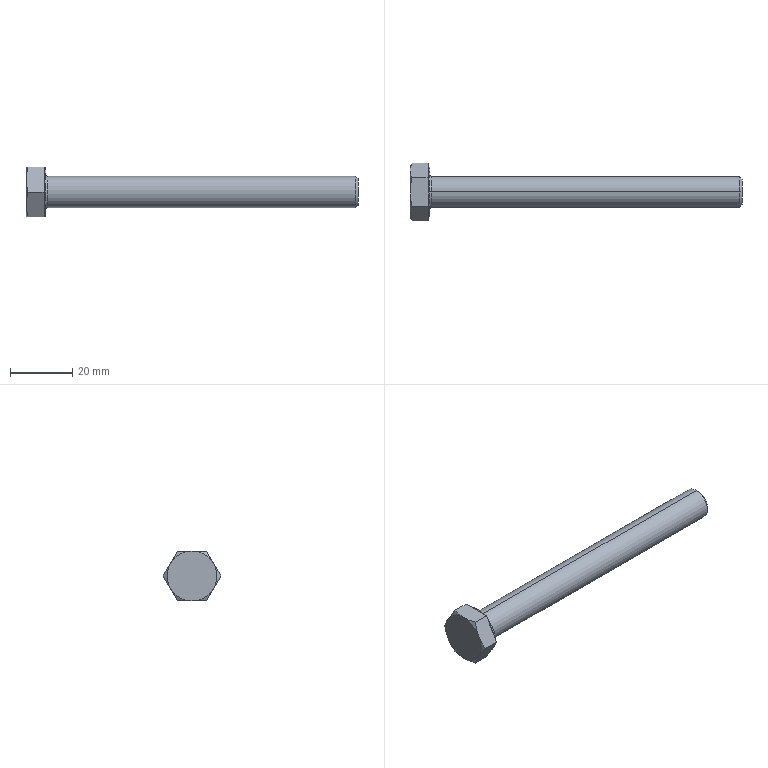Part | STEP file | Microwave Drying Flat Conveyor-hex screw gradeab_din_DIN EN 24017 - M10 x 100-N_Default | 1 solid | 29 faces | box 106.4 x 18.475 x 16 mm | volume 9247 mm3 | plane 15 | cone 8 | cylinder 4 | spline 2 | commonest cylinder face diameters 10 x2 16 x2
STEP:
#1=CARTESIAN_POINT('',(6.4,0.,5.4));
#2=VERTEX_POINT('',#1);
#3=CARTESIAN_POINT('',(6.4,0.,-5.4));
#4=VERTEX_POINT('',#3);
#5=CARTESIAN_POINT('',(6.4,0.,5.4));
#6=CARTESIAN_POINT('',(6.4,0.1651,5.4));
#7=CARTESIAN_POINT('',(6.4,0.4117,5.389));
#8=CARTESIAN_POINT('',(6.4,0.6977,5.356));
#9=CARTESIAN_POINT('',(6.4,0.8403,5.334));
#10=CARTESIAN_POINT('',(6.4,0.9013,5.324));
#11=CARTESIAN_POINT('',(6.4,0.942,5.317));
#12=CARTESIAN_POINT('',(6.4,0.9611,5.314));
#13=CARTESIAN_POINT('',(6.4,1.155,5.278));
#14=CARTESIAN_POINT('',(6.4,1.409,5.218));
#15=CARTESIAN_POINT('',(6.4,1.7,5.127));
#16=CARTESIAN_POINT('',(6.4,1.824,5.083));
#17=CARTESIAN_POINT('',(6.4,1.906,5.053));
#18=CARTESIAN_POINT('',(6.4,1.945,5.038));
#19=CARTESIAN_POINT('',(6.4,2.157,4.954));
#20=CARTESIAN_POINT('',(6.4,2.405,4.841));
#21=CARTESIAN_POINT('',(6.4,2.644,4.709));
#22=CARTESIAN_POINT('',(6.4,2.801,4.618));
#23=CARTESIAN_POINT('',(6.4,2.877,4.571));
#24=CARTESIAN_POINT('',(6.4,3.267,4.316));
#25=CARTESIAN_POINT('',(6.4,3.555,4.082));
#26=CARTESIAN_POINT('',(6.4,3.95,3.687));
#27=CARTESIAN_POINT('',(6.4,4.137,3.48));
#28=CARTESIAN_POINT('',(6.4,4.306,3.26));
#29=CARTESIAN_POINT('',(6.4,4.416,3.11));
#30=CARTESIAN_POINT('',(6.4,4.47,3.031));
#31=CARTESIAN_POINT('',(6.4,4.62,2.802));
#32=CARTESIAN_POINT('',(6.4,4.757,2.567));
#33=CARTESIAN_POINT('',(6.4,4.896,2.281));
#34=CARTESIAN_POINT('',(6.4,4.951,2.156));
#35=CARTESIAN_POINT('',(6.4,4.987,2.072));
#36=CARTESIAN_POINT('',(6.4,5.005,2.028));
#37=CARTESIAN_POINT('',(6.4,5.085,1.825));
#38=CARTESIAN_POINT('',(6.4,5.17,1.577));
#39=CARTESIAN_POINT('',(6.4,5.247,1.282));
#40=CARTESIAN_POINT('',(6.4,5.28,1.133));
#41=CARTESIAN_POINT('',(6.4,5.293,1.069));
#42=CARTESIAN_POINT('',(6.4,5.302,1.026));
#43=CARTESIAN_POINT('',(6.4,5.306,1.003));
#44=CARTESIAN_POINT('',(6.4,5.37,0.6582));
#45=CARTESIAN_POINT('',(6.4,5.4,0.3299));
#46=CARTESIAN_POINT('',(6.4,5.4,-0.165));
#47=CARTESIAN_POINT('',(6.4,5.389,-0.4115));
#48=CARTESIAN_POINT('',(6.4,5.356,-0.6976));
#49=CARTESIAN_POINT('',(6.4,5.335,-0.8402));
#50=CARTESIAN_POINT('',(6.4,5.324,-0.9013));
#51=CARTESIAN_POINT('',(6.4,5.317,-0.9419));
#52=CARTESIAN_POINT('',(6.4,5.314,-0.9611));
#53=CARTESIAN_POINT('',(6.4,5.278,-1.155));
#54=CARTESIAN_POINT('',(6.4,5.218,-1.409));
#55=CARTESIAN_POINT('',(6.4,5.127,-1.7));
#56=CARTESIAN_POINT('',(6.4,5.083,-1.824));
#57=CARTESIAN_POINT('',(6.4,5.053,-1.906));
#58=CARTESIAN_POINT('',(6.4,5.038,-1.945));
#59=CARTESIAN_POINT('',(6.4,4.954,-2.157));
#60=CARTESIAN_POINT('',(6.4,4.841,-2.405));
#61=CARTESIAN_POINT('',(6.4,4.709,-2.644));
#62=CARTESIAN_POINT('',(6.4,4.618,-2.801));
#63=CARTESIAN_POINT('',(6.4,4.571,-2.877));
#64=CARTESIAN_POINT('',(6.4,4.316,-3.267));
#65=CARTESIAN_POINT('',(6.4,4.082,-3.555));
#66=CARTESIAN_POINT('',(6.4,3.687,-3.95));
#67=CARTESIAN_POINT('',(6.4,3.48,-4.137));
#68=CARTESIAN_POINT('',(6.4,3.26,-4.306));
#69=CARTESIAN_POINT('',(6.4,3.11,-4.416));
#70=CARTESIAN_POINT('',(6.4,3.031,-4.47));
#71=CARTESIAN_POINT('',(6.4,2.802,-4.62));
#72=CARTESIAN_POINT('',(6.4,2.567,-4.757));
#73=CARTESIAN_POINT('',(6.4,2.281,-4.896));
#74=CARTESIAN_POINT('',(6.4,2.156,-4.951));
#75=CARTESIAN_POINT('',(6.4,2.072,-4.987));
#76=CARTESIAN_POINT('',(6.4,2.028,-5.005));
#77=CARTESIAN_POINT('',(6.4,1.825,-5.085));
#78=CARTESIAN_POINT('',(6.4,1.577,-5.17));
#79=CARTESIAN_POINT('',(6.4,1.282,-5.247));
#80=CARTESIAN_POINT('',(6.4,1.133,-5.28));
#81=CARTESIAN_POINT('',(6.4,1.069,-5.293));
#82=CARTESIAN_POINT('',(6.4,1.026,-5.302));
#83=CARTESIAN_POINT('',(6.4,1.003,-5.306));
#84=CARTESIAN_POINT('',(6.4,0.658,-5.37));
#85=CARTESIAN_POINT('',(6.4,0.3305,-5.4));
#86=CARTESIAN_POINT('',(6.4,0.,-5.4));
#87=B_SPLINE_CURVE_WITH_KNOTS('',3,(#5,#6,#7,#8,#9,#10,#11,#12,#13,#14,#15,#16,#17,#18,#19,#20,#21,#22,#23,#24,#25,#26,#27,#28,#29,#30,#31,#32,#33,#34,#35,#36,#37,#38,#39,#40,#41,#42,#43,#44,#45,#46,#47,#48,#49,#50,#51,#52,#53,#54,#55,#56,#57,#58,#59,#60,#61,#62,#63,#64,#65,#66,#67,#68,#69,#70,#71,#72,#73,#74,#75,#76,#77,#78,#79,#80,#81,#82,#83,#84,#85,#86),.UNSPECIFIED.,.F.,.F.,(4,1,1,1,2,2,1,1,2,2,1,2,2,2,1,2,2,1,1,2,2,1,1,1,2,2,2,1,1,1,2,2,1,1,2,2,1,2,2,2,1,2,2,1,1,2,2,1,1,1,2,2,4),(0.,0.03125,0.04687,0.05469,0.05859,0.0625,0.09375,0.1094,0.1172,0.125,0.1562,0.1719,0.1875,0.25,0.2812,0.2969,0.3125,0.3437,0.3594,0.3672,0.375,0.4062,0.4219,0.4297,0.4336,0.4375,0.5,0.5312,0.5469,0.5547,0.5586,0.5625,0.5937,0.6094,0.6172,0.625,0.6562,0.6719,0.6875,0.75,0.7812,0.7969,0.8125,0.8437,0.8594,0.8672,0.875,0.9062,0.9219,0.9297,0.9336,0.9375,1.),.UNSPECIFIED.);
#88=EDGE_CURVE('',#2,#4,#87,.T.);
#89=ORIENTED_EDGE('',*,*,#88,.F.);
#90=CARTESIAN_POINT('',(6.8,0.,5.));
#91=VERTEX_POINT('',#90);
#92=CARTESIAN_POINT('',(6.8,0.,5.4));
#93=DIRECTION('',(0.,-1.,0.));
#94=DIRECTION('',(0.,0.,1.));
#95=AXIS2_PLACEMENT_3D('',#92,#93,#94);
#96=CIRCLE('',#95,0.4);
#97=EDGE_CURVE('',#2,#91,#96,.T.);
#98=ORIENTED_EDGE('',*,*,#97,.T.);
#99=CARTESIAN_POINT('',(6.8,0.,-5.));
#100=VERTEX_POINT('',#99);
#101=CARTESIAN_POINT('',(6.8,0.,0.));
#102=DIRECTION('',(1.,0.,0.));
#103=DIRECTION('',(0.,0.,1.));
#104=AXIS2_PLACEMENT_3D('',#101,#102,#103);
#105=CIRCLE('',#104,5.);
#106=EDGE_CURVE('',#100,#91,#105,.T.);
#107=ORIENTED_EDGE('',*,*,#106,.F.);
#108=CARTESIAN_POINT('',(6.8,0.,-5.4));
#109=DIRECTION('',(0.,1.,0.));
#110=DIRECTION('',(0.,0.,-1.));
#111=AXIS2_PLACEMENT_3D('',#108,#109,#110);
#112=CIRCLE('',#111,0.4);
#113=EDGE_CURVE('',#4,#100,#112,.T.);
#114=ORIENTED_EDGE('',*,*,#113,.F.);
#115=EDGE_LOOP('',(#89,#98,#107,#114));
#116=FACE_OUTER_BOUND('',#115,.T.);
#117=CARTESIAN_POINT('',(6.4,0.,-5.4));
#118=CARTESIAN_POINT('',(6.4,10.8,-5.4));
#119=CARTESIAN_POINT('',(6.4,10.8,5.4));
#120=CARTESIAN_POINT('',(6.4,0.,5.4));
#121=CARTESIAN_POINT('',(6.4,0.,-5.166));
#122=CARTESIAN_POINT('',(6.4,10.331,-5.166));
#123=CARTESIAN_POINT('',(6.4,10.331,5.166));
#124=CARTESIAN_POINT('',(6.4,0.,5.166));
#125=CARTESIAN_POINT('',(6.566,0.,-5.));
#126=CARTESIAN_POINT('',(6.566,10.,-5.));
#127=CARTESIAN_POINT('',(6.566,10.,5.));
#128=CARTESIAN_POINT('',(6.566,0.,5.));
#129=CARTESIAN_POINT('',(6.8,0.,-5.));
#130=CARTESIAN_POINT('',(6.8,10.,-5.));
#131=CARTESIAN_POINT('',(6.8,10.,5.));
#132=CARTESIAN_POINT('',(6.8,0.,5.));
#133=(BOUNDED_SURFACE()B_SPLINE_SURFACE(3,3,((#117,#118,#119,#120),(#121,#122,#123,#124),(#125,#126,#127,#128),(#129,#130,#131,#132)),.UNSPECIFIED.,.F.,.F.,.F.)B_SPLINE_SURFACE_WITH_KNOTS((4,4),(4,4),(0.,1.),(0.,1.),.UNSPECIFIED.)GEOMETRIC_REPRESENTATION_ITEM()RATIONAL_B_SPLINE_SURFACE(((1.,0.3333,0.3333,1.),(0.8047,0.2682,0.2682,0.8047),(0.8047,0.2682,0.2682,0.8047),(1.,0.3333,0.3333,1.)))REPRESENTATION_ITEM('')SURFACE());
#134=ADVANCED_FACE('',(#116),#133,.F.);
#135=CARTESIAN_POINT('',(105.572,0.,5.));
#136=VERTEX_POINT('',#135);
#137=CARTESIAN_POINT('',(105.572,0.,-5.));
#138=VERTEX_POINT('',#137);
#139=CARTESIAN_POINT('',(105.572,0.,0.));
#140=DIRECTION('',(-1.,0.,0.));
#141=DIRECTION('',(0.,0.,1.));
#142=AXIS2_PLACEMENT_3D('',#139,#140,#141);
#143=CIRCLE('',#142,5.);
#144=EDGE_CURVE('',#136,#138,#143,.T.);
#145=ORIENTED_EDGE('',*,*,#144,.T.);
#146=CARTESIAN_POINT('',(0.,0.,-5.));
#147=DIRECTION('',(-1.,0.,0.));
#148=VECTOR('',#147,1000.);
#149=LINE('',#146,#148);
#150=EDGE_CURVE('',#138,#100,#149,.T.);
#151=ORIENTED_EDGE('',*,*,#150,.T.);
#152=ORIENTED_EDGE('',*,*,#106,.T.);
#153=CARTESIAN_POINT('',(0.,0.,5.));
#154=DIRECTION('',(-1.,0.,0.));
#155=VECTOR('',#154,1000.);
#156=LINE('',#153,#155);
#157=EDGE_CURVE('',#136,#91,#156,.T.);
#158=ORIENTED_EDGE('',*,*,#157,.F.);
#159=EDGE_LOOP('',(#145,#151,#152,#158));
#160=FACE_OUTER_BOUND('',#159,.T.);
#161=CARTESIAN_POINT('',(0.,0.,0.));
#162=DIRECTION('',(-1.,0.,0.));
#163=DIRECTION('',(0.,0.,1.));
#164=AXIS2_PLACEMENT_3D('',#161,#162,#163);
#165=CYLINDRICAL_SURFACE('',#164,5.);
#166=ADVANCED_FACE('',(#160),#165,.T.);
#167=CARTESIAN_POINT('',(106.4,0.,4.172));
#168=VERTEX_POINT('',#167);
#169=CARTESIAN_POINT('',(106.4,0.,-4.172));
#170=VERTEX_POINT('',#169);
#171=CARTESIAN_POINT('',(106.4,0.,0.));
#172=DIRECTION('',(-1.,0.,0.));
#173=DIRECTION('',(0.,0.,1.));
#174=AXIS2_PLACEMENT_3D('',#171,#172,#173);
#175=CIRCLE('',#174,4.172);
#176=EDGE_CURVE('',#168,#170,#175,.T.);
#177=ORIENTED_EDGE('',*,*,#176,.T.);
#178=CARTESIAN_POINT('',(105.572,0.,-5.));
#179=DIRECTION('',(-0.7071,0.,-0.7071));
#180=VECTOR('',#179,1000.);
#181=LINE('',#178,#180);
#182=EDGE_CURVE('',#170,#138,#181,.T.);
#183=ORIENTED_EDGE('',*,*,#182,.T.);
#184=ORIENTED_EDGE('',*,*,#144,.F.);
#185=CARTESIAN_POINT('',(105.572,0.,5.));
#186=DIRECTION('',(-0.7071,0.,0.7071));
#187=VECTOR('',#186,1000.);
#188=LINE('',#185,#187);
#189=EDGE_CURVE('',#168,#136,#188,.T.);
#190=ORIENTED_EDGE('',*,*,#189,.F.);
#191=EDGE_LOOP('',(#177,#183,#184,#190));
#192=FACE_OUTER_BOUND('',#191,.T.);
#193=CARTESIAN_POINT('',(105.572,0.,0.));
#194=DIRECTION('',(-1.,0.,0.));
#195=DIRECTION('',(0.,0.,1.));
#196=AXIS2_PLACEMENT_3D('',#193,#194,#195);
#197=CONICAL_SURFACE('',#196,5.,0.7854);
#198=ADVANCED_FACE('',(#192),#197,.T.);
#199=CARTESIAN_POINT('',(6.4,0.,-8.));
#200=VERTEX_POINT('',#199);
#201=CARTESIAN_POINT('',(6.4,0.,8.));
#202=VERTEX_POINT('',#201);
#203=CARTESIAN_POINT('',(6.4,0.,0.));
#204=DIRECTION('',(1.,0.,0.));
#205=DIRECTION('',(0.,0.,1.));
#206=AXIS2_PLACEMENT_3D('',#203,#204,#205);
#207=CIRCLE('',#206,8.);
#208=EDGE_CURVE('',#200,#202,#207,.T.);
#209=ORIENTED_EDGE('',*,*,#208,.F.);
#210=CARTESIAN_POINT('',(5.8,0.,-8.));
#211=VERTEX_POINT('',#210);
#212=CARTESIAN_POINT('',(0.,0.,-8.));
#213=DIRECTION('',(-1.,0.,0.));
#214=VECTOR('',#213,1000.);
#215=LINE('',#212,#214);
#216=EDGE_CURVE('',#200,#211,#215,.T.);
#217=ORIENTED_EDGE('',*,*,#216,.T.);
#218=CARTESIAN_POINT('',(5.8,6.928,-4.));
#219=VERTEX_POINT('',#218);
#220=CARTESIAN_POINT('',(5.8,0.,0.));
#221=DIRECTION('',(1.,0.,0.));
#222=DIRECTION('',(0.,0.,1.));
#223=AXIS2_PLACEMENT_3D('',#220,#221,#222);
#224=CIRCLE('',#223,8.);
#225=EDGE_CURVE('',#211,#219,#224,.T.);
#226=ORIENTED_EDGE('',*,*,#225,.T.);
#227=CARTESIAN_POINT('',(5.8,6.928,4.));
#228=VERTEX_POINT('',#227);
#229=CARTESIAN_POINT('',(5.8,0.,0.));
#230=DIRECTION('',(1.,0.,0.));
#231=DIRECTION('',(0.,0.,1.));
#232=AXIS2_PLACEMENT_3D('',#229,#230,#231);
#233=CIRCLE('',#232,8.);
#234=EDGE_CURVE('',#219,#228,#233,.T.);
#235=ORIENTED_EDGE('',*,*,#234,.T.);
#236=CARTESIAN_POINT('',(5.8,0.,8.));
#237=VERTEX_POINT('',#236);
#238=CARTESIAN_POINT('',(5.8,0.,0.));
#239=DIRECTION('',(1.,0.,0.));
#240=DIRECTION('',(0.,0.,1.));
#241=AXIS2_PLACEMENT_3D('',#238,#239,#240);
#242=CIRCLE('',#241,8.);
#243=EDGE_CURVE('',#228,#237,#242,.T.);
#244=ORIENTED_EDGE('',*,*,#243,.T.);
#245=CARTESIAN_POINT('',(0.,0.,8.));
#246=DIRECTION('',(-1.,0.,0.));
#247=VECTOR('',#246,1000.);
#248=LINE('',#245,#247);
#249=EDGE_CURVE('',#202,#237,#248,.T.);
#250=ORIENTED_EDGE('',*,*,#249,.F.);
#251=EDGE_LOOP('',(#209,#217,#226,#235,#244,#250));
#252=FACE_OUTER_BOUND('',#251,.T.);
#253=CARTESIAN_POINT('',(0.,0.,0.));
#254=DIRECTION('',(-1.,0.,0.));
#255=DIRECTION('',(0.,0.,1.));
#256=AXIS2_PLACEMENT_3D('',#253,#254,#255);
#257=CYLINDRICAL_SURFACE('',#256,8.);
#258=ADVANCED_FACE('',(#252),#257,.T.);
#259=ORIENTED_EDGE('',*,*,#150,.F.);
#260=CARTESIAN_POINT('',(105.572,0.,0.));
#261=DIRECTION('',(-1.,0.,0.));
#262=DIRECTION('',(0.,0.,1.));
#263=AXIS2_PLACEMENT_3D('',#260,#261,#262);
#264=CIRCLE('',#263,5.);
#265=EDGE_CURVE('',#138,#136,#264,.T.);
#266=ORIENTED_EDGE('',*,*,#265,.T.);
#267=ORIENTED_EDGE('',*,*,#157,.T.);
#268=CARTESIAN_POINT('',(6.8,0.,0.));
#269=DIRECTION('',(1.,0.,0.));
#270=DIRECTION('',(0.,0.,1.));
#271=AXIS2_PLACEMENT_3D('',#268,#269,#270);
#272=CIRCLE('',#271,5.);
#273=EDGE_CURVE('',#91,#100,#272,.T.);
#274=ORIENTED_EDGE('',*,*,#273,.T.);
#275=EDGE_LOOP('',(#259,#266,#267,#274));
#276=FACE_OUTER_BOUND('',#275,.T.);
#277=CARTESIAN_POINT('',(0.,0.,0.));
#278=DIRECTION('',(-1.,0.,0.));
#279=DIRECTION('',(0.,0.,1.));
#280=AXIS2_PLACEMENT_3D('',#277,#278,#279);
#281=CYLINDRICAL_SURFACE('',#280,5.);
#282=ADVANCED_FACE('',(#276),#281,.T.);
#283=ORIENTED_EDGE('',*,*,#97,.F.);
#284=CARTESIAN_POINT('',(6.4,0.,-5.4));
#285=CARTESIAN_POINT('',(6.4,-0.1651,-5.4));
#286=CARTESIAN_POINT('',(6.4,-0.4117,-5.389));
#287=CARTESIAN_POINT('',(6.4,-0.6977,-5.356));
#288=CARTESIAN_POINT('',(6.4,-0.8403,-5.334));
#289=CARTESIAN_POINT('',(6.4,-0.9013,-5.324));
#290=CARTESIAN_POINT('',(6.4,-0.942,-5.317));
#291=CARTESIAN_POINT('',(6.4,-0.9611,-5.314));
#292=CARTESIAN_POINT('',(6.4,-1.155,-5.278));
#293=CARTESIAN_POINT('',(6.4,-1.409,-5.218));
#294=CARTESIAN_POINT('',(6.4,-1.7,-5.127));
#295=CARTESIAN_POINT('',(6.4,-1.824,-5.083));
#296=CARTESIAN_POINT('',(6.4,-1.906,-5.053));
#297=CARTESIAN_POINT('',(6.4,-1.945,-5.038));
#298=CARTESIAN_POINT('',(6.4,-2.157,-4.954));
#299=CARTESIAN_POINT('',(6.4,-2.405,-4.841));
#300=CARTESIAN_POINT('',(6.4,-2.644,-4.709));
#301=CARTESIAN_POINT('',(6.4,-2.801,-4.618));
#302=CARTESIAN_POINT('',(6.4,-2.877,-4.571));
#303=CARTESIAN_POINT('',(6.4,-3.267,-4.316));
#304=CARTESIAN_POINT('',(6.4,-3.555,-4.082));
#305=CARTESIAN_POINT('',(6.4,-3.95,-3.687));
#306=CARTESIAN_POINT('',(6.4,-4.137,-3.48));
#307=CARTESIAN_POINT('',(6.4,-4.306,-3.26));
#308=CARTESIAN_POINT('',(6.4,-4.416,-3.11));
#309=CARTESIAN_POINT('',(6.4,-4.47,-3.031));
#310=CARTESIAN_POINT('',(6.4,-4.62,-2.802));
#311=CARTESIAN_POINT('',(6.4,-4.757,-2.567));
#312=CARTESIAN_POINT('',(6.4,-4.896,-2.281));
#313=CARTESIAN_POINT('',(6.4,-4.951,-2.156));
#314=CARTESIAN_POINT('',(6.4,-4.987,-2.072));
#315=CARTESIAN_POINT('',(6.4,-5.005,-2.028));
#316=CARTESIAN_POINT('',(6.4,-5.085,-1.825));
#317=CARTESIAN_POINT('',(6.4,-5.17,-1.577));
#318=CARTESIAN_POINT('',(6.4,-5.247,-1.282));
#319=CARTESIAN_POINT('',(6.4,-5.28,-1.133));
#320=CARTESIAN_POINT('',(6.4,-5.293,-1.069));
#321=CARTESIAN_POINT('',(6.4,-5.302,-1.026));
#322=CARTESIAN_POINT('',(6.4,-5.306,-1.003));
#323=CARTESIAN_POINT('',(6.4,-5.37,-0.6582));
#324=CARTESIAN_POINT('',(6.4,-5.4,-0.3299));
#325=CARTESIAN_POINT('',(6.4,-5.4,0.165));
#326=CARTESIAN_POINT('',(6.4,-5.389,0.4115));
#327=CARTESIAN_POINT('',(6.4,-5.356,0.6976));
#328=CARTESIAN_POINT('',(6.4,-5.335,0.8402));
#329=CARTESIAN_POINT('',(6.4,-5.324,0.9013));
#330=CARTESIAN_POINT('',(6.4,-5.317,0.9419));
#331=CARTESIAN_POINT('',(6.4,-5.314,0.9611));
#332=CARTESIAN_POINT('',(6.4,-5.278,1.155));
#333=CARTESIAN_POINT('',(6.4,-5.218,1.409));
#334=CARTESIAN_POINT('',(6.4,-5.127,1.7));
#335=CARTESIAN_POINT('',(6.4,-5.083,1.824));
#336=CARTESIAN_POINT('',(6.4,-5.053,1.906));
#337=CARTESIAN_POINT('',(6.4,-5.038,1.945));
#338=CARTESIAN_POINT('',(6.4,-4.954,2.157));
#339=CARTESIAN_POINT('',(6.4,-4.841,2.405));
#340=CARTESIAN_POINT('',(6.4,-4.709,2.644));
#341=CARTESIAN_POINT('',(6.4,-4.618,2.801));
#342=CARTESIAN_POINT('',(6.4,-4.571,2.877));
#343=CARTESIAN_POINT('',(6.4,-4.316,3.267));
#344=CARTESIAN_POINT('',(6.4,-4.082,3.555));
#345=CARTESIAN_POINT('',(6.4,-3.687,3.95));
#346=CARTESIAN_POINT('',(6.4,-3.48,4.137));
#347=CARTESIAN_POINT('',(6.4,-3.26,4.306));
#348=CARTESIAN_POINT('',(6.4,-3.11,4.416));
#349=CARTESIAN_POINT('',(6.4,-3.031,4.47));
#350=CARTESIAN_POINT('',(6.4,-2.802,4.62));
#351=CARTESIAN_POINT('',(6.4,-2.567,4.757));
#352=CARTESIAN_POINT('',(6.4,-2.281,4.896));
#353=CARTESIAN_POINT('',(6.4,-2.156,4.951));
#354=CARTESIAN_POINT('',(6.4,-2.072,4.987));
#355=CARTESIAN_POINT('',(6.4,-2.028,5.005));
#356=CARTESIAN_POINT('',(6.4,-1.825,5.085));
#357=CARTESIAN_POINT('',(6.4,-1.577,5.17));
#358=CARTESIAN_POINT('',(6.4,-1.282,5.247));
#359=CARTESIAN_POINT('',(6.4,-1.133,5.28));
#360=CARTESIAN_POINT('',(6.4,-1.069,5.293));
#361=CARTESIAN_POINT('',(6.4,-1.026,5.302));
#362=CARTESIAN_POINT('',(6.4,-1.003,5.306));
#363=CARTESIAN_POINT('',(6.4,-0.658,5.37));
#364=CARTESIAN_POINT('',(6.4,-0.3305,5.4));
#365=CARTESIAN_POINT('',(6.4,0.,5.4));
#366=B_SPLINE_CURVE_WITH_KNOTS('',3,(#284,#285,#286,#287,#288,#289,#290,#291,#292,#293,#294,#295,#296,#297,#298,#299,#300,#301,#302,#303,#304,#305,#306,#307,#308,#309,#310,#311,#312,#313,#314,#315,#316,#317,#318,#319,#320,#321,#322,#323,#324,#325,#326,#327,#328,#329,#330,#331,#332,#333,#334,#335,#336,#337,#338,#339,#340,#341,#342,#343,#344,#345,#346,#347,#348,#349,#350,#351,#352,#353,#354,#355,#356,#357,#358,#359,#360,#361,#362,#363,#364,#365),.UNSPECIFIED.,.F.,.F.,(4,1,1,1,2,2,1,1,2,2,1,2,2,2,1,2,2,1,1,2,2,1,1,1,2,2,2,1,1,1,2,2,1,1,2,2,1,2,2,2,1,2,2,1,1,2,2,1,1,1,2,2,4),(0.,0.03125,0.04687,0.05469,0.05859,0.0625,0.09375,0.1094,0.1172,0.125,0.1562,0.1719,0.1875,0.25,0.2812,0.2969,0.3125,0.3437,0.3594,0.3672,0.375,0.4062,0.4219,0.4297,0.4336,0.4375,0.5,0.5312,0.5469,0.5547,0.5586,0.5625,0.5937,0.6094,0.6172,0.625,0.6562,0.6719,0.6875,0.75,0.7812,0.7969,0.8125,0.8437,0.8594,0.8672,0.875,0.9062,0.9219,0.9297,0.9336,0.9375,1.),.UNSPECIFIED.);
#367=EDGE_CURVE('',#4,#2,#366,.T.);
#368=ORIENTED_EDGE('',*,*,#367,.F.);
#369=ORIENTED_EDGE('',*,*,#113,.T.);
#370=ORIENTED_EDGE('',*,*,#273,.F.);
#371=EDGE_LOOP('',(#283,#368,#369,#370));
#372=FACE_OUTER_BOUND('',#371,.T.);
#373=CARTESIAN_POINT('',(6.4,0.,5.4));
#374=CARTESIAN_POINT('',(6.4,-10.8,5.4));
#375=CARTESIAN_POINT('',(6.4,-10.8,-5.4));
#376=CARTESIAN_POINT('',(6.4,0.,-5.4));
#377=CARTESIAN_POINT('',(6.4,0.,5.166));
#378=CARTESIAN_POINT('',(6.4,-10.331,5.166));
#379=CARTESIAN_POINT('',(6.4,-10.331,-5.166));
#380=CARTESIAN_POINT('',(6.4,0.,-5.166));
#381=CARTESIAN_POINT('',(6.566,0.,5.));
#382=CARTESIAN_POINT('',(6.566,-10.,5.));
#383=CARTESIAN_POINT('',(6.566,-10.,-5.));
#384=CARTESIAN_POINT('',(6.566,0.,-5.));
#385=CARTESIAN_POINT('',(6.8,0.,5.));
#386=CARTESIAN_POINT('',(6.8,-10.,5.));
#387=CARTESIAN_POINT('',(6.8,-10.,-5.));
#388=CARTESIAN_POINT('',(6.8,0.,-5.));
#389=(BOUNDED_SURFACE()B_SPLINE_SURFACE(3,3,((#373,#374,#375,#376),(#377,#378,#379,#380),(#381,#382,#383,#384),(#385,#386,#387,#388)),.UNSPECIFIED.,.F.,.F.,.T.)B_SPLINE_SURFACE_WITH_KNOTS((4,4),(4,4),(0.,1.),(0.,1.),.UNSPECIFIED.)GEOMETRIC_REPRESENTATION_ITEM()RATIONAL_B_SPLINE_SURFACE(((1.,0.3333,0.3333,1.),(0.8047,0.2682,0.2682,0.8047),(0.8047,0.2682,0.2682,0.8047),(1.,0.3333,0.3333,1.)))REPRESENTATION_ITEM('')SURFACE());
#390=ADVANCED_FACE('',(#372),#389,.F.);
#391=ORIENTED_EDGE('',*,*,#182,.F.);
#392=CARTESIAN_POINT('',(106.4,0.,0.));
#393=DIRECTION('',(-1.,0.,0.));
#394=DIRECTION('',(0.,0.,1.));
#395=AXIS2_PLACEMENT_3D('',#392,#393,#394);
#396=CIRCLE('',#395,4.172);
#397=EDGE_CURVE('',#170,#168,#396,.T.);
#398=ORIENTED_EDGE('',*,*,#397,.T.);
#399=ORIENTED_EDGE('',*,*,#189,.T.);
#400=ORIENTED_EDGE('',*,*,#265,.F.);
#401=EDGE_LOOP('',(#391,#398,#399,#400));
#402=FACE_OUTER_BOUND('',#401,.T.);
#403=CARTESIAN_POINT('',(105.572,0.,0.));
#404=DIRECTION('',(-1.,0.,0.));
#405=DIRECTION('',(0.,0.,1.));
#406=AXIS2_PLACEMENT_3D('',#403,#404,#405);
#407=CONICAL_SURFACE('',#406,5.,0.7854);
#408=ADVANCED_FACE('',(#402),#407,.T.);
#409=CARTESIAN_POINT('',(6.4,0.,0.));
#410=DIRECTION('',(1.,0.,0.));
#411=DIRECTION('',(0.,0.,1.));
#412=AXIS2_PLACEMENT_3D('',#409,#410,#411);
#413=CIRCLE('',#412,8.);
#414=EDGE_CURVE('',#202,#200,#413,.T.);
#415=ORIENTED_EDGE('',*,*,#414,.T.);
#416=ORIENTED_EDGE('',*,*,#208,.T.);
#417=EDGE_LOOP('',(#415,#416));
#418=FACE_OUTER_BOUND('',#417,.T.);
#419=ORIENTED_EDGE('',*,*,#367,.T.);
#420=ORIENTED_EDGE('',*,*,#88,.T.);
#421=EDGE_LOOP('',(#419,#420));
#422=FACE_BOUND('',#421,.T.);
#423=CARTESIAN_POINT('',(6.4,9.238,0.));
#424=DIRECTION('',(1.,0.,0.));
#425=DIRECTION('',(0.,0.,-1.));
#426=AXIS2_PLACEMENT_3D('',#423,#424,#425);
#427=PLANE('',#426);
#428=ADVANCED_FACE('',(#418,#422),#427,.T.);
#429=ORIENTED_EDGE('',*,*,#176,.F.);
#430=ORIENTED_EDGE('',*,*,#397,.F.);
#431=EDGE_LOOP('',(#429,#430));
#432=FACE_OUTER_BOUND('',#431,.T.);
#433=CARTESIAN_POINT('',(106.4,0.,0.));
#434=DIRECTION('',(-1.,0.,0.));
#435=DIRECTION('',(0.,0.,1.));
#436=AXIS2_PLACEMENT_3D('',#433,#434,#435);
#437=PLANE('',#436);
#438=ADVANCED_FACE('',(#432),#437,.F.);
#439=ORIENTED_EDGE('',*,*,#216,.F.);
#440=ORIENTED_EDGE('',*,*,#414,.F.);
#441=ORIENTED_EDGE('',*,*,#249,.T.);
#442=CARTESIAN_POINT('',(5.8,-6.928,4.));
#443=VERTEX_POINT('',#442);
#444=CARTESIAN_POINT('',(5.8,0.,0.));
#445=DIRECTION('',(1.,0.,0.));
#446=DIRECTION('',(0.,0.,1.));
#447=AXIS2_PLACEMENT_3D('',#444,#445,#446);
#448=CIRCLE('',#447,8.);
#449=EDGE_CURVE('',#237,#443,#448,.T.);
#450=ORIENTED_EDGE('',*,*,#449,.T.);
#451=CARTESIAN_POINT('',(5.8,-6.928,-4.));
#452=VERTEX_POINT('',#451);
#453=CARTESIAN_POINT('',(5.8,0.,0.));
#454=DIRECTION('',(1.,0.,0.));
#455=DIRECTION('',(0.,0.,1.));
#456=AXIS2_PLACEMENT_3D('',#453,#454,#455);
#457=CIRCLE('',#456,8.);
#458=EDGE_CURVE('',#443,#452,#457,.T.);
#459=ORIENTED_EDGE('',*,*,#458,.T.);
#460=CARTESIAN_POINT('',(5.8,0.,0.));
#461=DIRECTION('',(1.,0.,0.));
#462=DIRECTION('',(0.,0.,1.));
#463=AXIS2_PLACEMENT_3D('',#460,#461,#462);
#464=CIRCLE('',#463,8.);
#465=EDGE_CURVE('',#452,#211,#464,.T.);
#466=ORIENTED_EDGE('',*,*,#465,.T.);
#467=EDGE_LOOP('',(#439,#440,#441,#450,#459,#466));
#468=FACE_OUTER_BOUND('',#467,.T.);
#469=CARTESIAN_POINT('',(0.,0.,0.));
#470=DIRECTION('',(-1.,0.,0.));
#471=DIRECTION('',(0.,0.,1.));
#472=AXIS2_PLACEMENT_3D('',#469,#470,#471);
#473=CYLINDRICAL_SURFACE('',#472,8.);
#474=ADVANCED_FACE('',(#468),#473,.T.);
#475=CARTESIAN_POINT('',(5.8,4.619,8.));
#476=VERTEX_POINT('',#475);
#477=CARTESIAN_POINT('',(5.8,8.,8.));
#478=DIRECTION('',(0.,-1.,0.));
#479=VECTOR('',#478,1000.);
#480=LINE('',#477,#479);
#481=EDGE_CURVE('',#476,#237,#480,.T.);
#482=ORIENTED_EDGE('',*,*,#481,.T.);
#483=ORIENTED_EDGE('',*,*,#243,.F.);
#484=CARTESIAN_POINT('',(5.8,6.928,4.));
#485=DIRECTION('',(0.,-0.5,0.866));
#486=VECTOR('',#485,1000.);
#487=LINE('',#484,#486);
#488=EDGE_CURVE('',#228,#476,#487,.T.);
#489=ORIENTED_EDGE('',*,*,#488,.T.);
#490=EDGE_LOOP('',(#482,#483,#489));
#491=FACE_OUTER_BOUND('',#490,.T.);
#492=CARTESIAN_POINT('',(5.8,8.,0.));
#493=DIRECTION('',(1.,0.,0.));
#494=DIRECTION('',(0.,0.,-1.));
#495=AXIS2_PLACEMENT_3D('',#492,#493,#494);
#496=PLANE('',#495);
#497=ADVANCED_FACE('',(#491),#496,.T.);
#498=CARTESIAN_POINT('',(5.8,9.238,0.));
#499=VERTEX_POINT('',#498);
#500=CARTESIAN_POINT('',(5.8,9.238,0.));
#501=DIRECTION('',(0.,-0.5,0.866));
#502=VECTOR('',#501,1000.);
#503=LINE('',#500,#502);
#504=EDGE_CURVE('',#499,#228,#503,.T.);
#505=ORIENTED_EDGE('',*,*,#504,.T.);
#506=ORIENTED_EDGE('',*,*,#234,.F.);
#507=CARTESIAN_POINT('',(5.8,6.928,-4.));
#508=DIRECTION('',(0.,0.5,0.866));
#509=VECTOR('',#508,1000.);
#510=LINE('',#507,#509);
#511=EDGE_CURVE('',#219,#499,#510,.T.);
#512=ORIENTED_EDGE('',*,*,#511,.T.);
#513=EDGE_LOOP('',(#505,#506,#512));
#514=FACE_OUTER_BOUND('',#513,.T.);
#515=CARTESIAN_POINT('',(5.8,8.,0.));
#516=DIRECTION('',(1.,0.,0.));
#517=DIRECTION('',(0.,0.,-1.));
#518=AXIS2_PLACEMENT_3D('',#515,#516,#517);
#519=PLANE('',#518);
#520=ADVANCED_FACE('',(#514),#519,.T.);
#521=ORIENTED_EDGE('',*,*,#225,.F.);
#522=CARTESIAN_POINT('',(5.8,4.619,-8.));
#523=VERTEX_POINT('',#522);
#524=CARTESIAN_POINT('',(5.8,8.,-8.));
#525=DIRECTION('',(0.,1.,0.));
#526=VECTOR('',#525,1000.);
#527=LINE('',#524,#526);
#528=EDGE_CURVE('',#211,#523,#527,.T.);
#529=ORIENTED_EDGE('',*,*,#528,.T.);
#530=CARTESIAN_POINT('',(5.8,4.619,-8.));
#531=DIRECTION('',(0.,0.5,0.866));
#532=VECTOR('',#531,1000.);
#533=LINE('',#530,#532);
#534=EDGE_CURVE('',#523,#219,#533,.T.);
#535=ORIENTED_EDGE('',*,*,#534,.T.);
#536=EDGE_LOOP('',(#521,#529,#535));
#537=FACE_OUTER_BOUND('',#536,.T.);
#538=CARTESIAN_POINT('',(5.8,8.,0.));
#539=DIRECTION('',(1.,0.,0.));
#540=DIRECTION('',(0.,0.,-1.));
#541=AXIS2_PLACEMENT_3D('',#538,#539,#540);
#542=PLANE('',#541);
#543=ADVANCED_FACE('',(#537),#542,.T.);
#544=CARTESIAN_POINT('',(5.8,-4.619,-8.));
#545=VERTEX_POINT('',#544);
#546=CARTESIAN_POINT('',(5.8,8.,-8.));
#547=DIRECTION('',(0.,1.,0.));
#548=VECTOR('',#547,1000.);
#549=LINE('',#546,#548);
#550=EDGE_CURVE('',#545,#211,#549,.T.);
#551=ORIENTED_EDGE('',*,*,#550,.T.);
#552=ORIENTED_EDGE('',*,*,#465,.F.);
#553=CARTESIAN_POINT('',(5.8,-6.928,-4.));
#554=DIRECTION('',(0.,0.5,-0.866));
#555=VECTOR('',#554,1000.);
#556=LINE('',#553,#555);
#557=EDGE_CURVE('',#452,#545,#556,.T.);
#558=ORIENTED_EDGE('',*,*,#557,.T.);
#559=EDGE_LOOP('',(#551,#552,#558));
#560=FACE_OUTER_BOUND('',#559,.T.);
#561=CARTESIAN_POINT('',(5.8,8.,0.));
#562=DIRECTION('',(1.,0.,0.));
#563=DIRECTION('',(0.,0.,-1.));
#564=AXIS2_PLACEMENT_3D('',#561,#562,#563);
#565=PLANE('',#564);
#566=ADVANCED_FACE('',(#560),#565,.T.);
#567=CARTESIAN_POINT('',(5.8,-9.238,0.));
#568=VERTEX_POINT('',#567);
#569=CARTESIAN_POINT('',(5.8,-9.238,0.));
#570=DIRECTION('',(0.,0.5,-0.866));
#571=VECTOR('',#570,1000.);
#572=LINE('',#569,#571);
#573=EDGE_CURVE('',#568,#452,#572,.T.);
#574=ORIENTED_EDGE('',*,*,#573,.T.);
#575=ORIENTED_EDGE('',*,*,#458,.F.);
#576=CARTESIAN_POINT('',(5.8,-6.928,4.));
#577=DIRECTION('',(0.,-0.5,-0.866));
#578=VECTOR('',#577,1000.);
#579=LINE('',#576,#578);
#580=EDGE_CURVE('',#443,#568,#579,.T.);
#581=ORIENTED_EDGE('',*,*,#580,.T.);
#582=EDGE_LOOP('',(#574,#575,#581));
#583=FACE_OUTER_BOUND('',#582,.T.);
#584=CARTESIAN_POINT('',(5.8,8.,0.));
#585=DIRECTION('',(1.,0.,0.));
#586=DIRECTION('',(0.,0.,-1.));
#587=AXIS2_PLACEMENT_3D('',#584,#585,#586);
#588=PLANE('',#587);
#589=ADVANCED_FACE('',(#583),#588,.T.);
#590=CARTESIAN_POINT('',(5.8,-4.619,8.));
#591=VERTEX_POINT('',#590);
#592=CARTESIAN_POINT('',(5.8,-4.619,8.));
#593=DIRECTION('',(0.,-0.5,-0.866));
#594=VECTOR('',#593,1000.);
#595=LINE('',#592,#594);
#596=EDGE_CURVE('',#591,#443,#595,.T.);
#597=ORIENTED_EDGE('',*,*,#596,.T.);
#598=ORIENTED_EDGE('',*,*,#449,.F.);
#599=CARTESIAN_POINT('',(5.8,8.,8.));
#600=DIRECTION('',(0.,-1.,0.));
#601=VECTOR('',#600,1000.);
#602=LINE('',#599,#601);
#603=EDGE_CURVE('',#237,#591,#602,.T.);
#604=ORIENTED_EDGE('',*,*,#603,.T.);
#605=EDGE_LOOP('',(#597,#598,#604));
#606=FACE_OUTER_BOUND('',#605,.T.);
#607=CARTESIAN_POINT('',(5.8,8.,0.));
#608=DIRECTION('',(1.,0.,0.));
#609=DIRECTION('',(0.,0.,-1.));
#610=AXIS2_PLACEMENT_3D('',#607,#608,#609);
#611=PLANE('',#610);
#612=ADVANCED_FACE('',(#606),#611,.T.);
#613=CARTESIAN_POINT('',(0.7145,4.619,8.));
#614=VERTEX_POINT('',#613);
#615=CARTESIAN_POINT('',(6.4,4.619,8.));
#616=DIRECTION('',(1.,0.,0.));
#617=VECTOR('',#616,1000.);
#618=LINE('',#615,#617);
#619=EDGE_CURVE('',#614,#476,#618,.T.);
#620=ORIENTED_EDGE('',*,*,#619,.F.);
#621=CARTESIAN_POINT('',(0.,0.,8.));
#622=VERTEX_POINT('',#621);
#623=CARTESIAN_POINT('',(0.,0.,8.));
#624=CARTESIAN_POINT('',(0.,0.7882,8.));
#625=CARTESIAN_POINT('',(0.06831,1.566,8.));
#626=CARTESIAN_POINT('',(0.3171,3.104,8.));
#627=CARTESIAN_POINT('',(0.4967,3.864,8.));
#628=CARTESIAN_POINT('',(0.7145,4.619,8.));
#629=B_SPLINE_CURVE_WITH_KNOTS('',3,(#623,#624,#625,#626,#627,#628),.UNSPECIFIED.,.F.,.F.,(4,2,4),(0.,0.002337,0.004674),.UNSPECIFIED.);
#630=EDGE_CURVE('',#622,#614,#629,.T.);
#631=ORIENTED_EDGE('',*,*,#630,.F.);
#632=CARTESIAN_POINT('',(0.7145,-4.619,8.));
#633=VERTEX_POINT('',#632);
#634=CARTESIAN_POINT('',(0.7145,-4.619,8.));
#635=CARTESIAN_POINT('',(0.4967,-3.864,8.));
#636=CARTESIAN_POINT('',(0.3171,-3.104,8.));
#637=CARTESIAN_POINT('',(0.06831,-1.566,8.));
#638=CARTESIAN_POINT('',(0.,-0.7882,8.));
#639=CARTESIAN_POINT('',(0.,0.,8.));
#640=B_SPLINE_CURVE_WITH_KNOTS('',3,(#634,#635,#636,#637,#638,#639),.UNSPECIFIED.,.F.,.F.,(4,2,4),(0.,0.002337,0.004674),.UNSPECIFIED.);
#641=EDGE_CURVE('',#633,#622,#640,.T.);
#642=ORIENTED_EDGE('',*,*,#641,.F.);
#643=CARTESIAN_POINT('',(6.4,-4.619,8.));
#644=DIRECTION('',(-1.,0.,0.));
#645=VECTOR('',#644,1000.);
#646=LINE('',#643,#645);
#647=EDGE_CURVE('',#591,#633,#646,.T.);
#648=ORIENTED_EDGE('',*,*,#647,.F.);
#649=ORIENTED_EDGE('',*,*,#603,.F.);
#650=ORIENTED_EDGE('',*,*,#481,.F.);
#651=EDGE_LOOP('',(#620,#631,#642,#648,#649,#650));
#652=FACE_OUTER_BOUND('',#651,.T.);
#653=CARTESIAN_POINT('',(6.4,4.619,8.));
#654=DIRECTION('',(0.,0.,-1.));
#655=DIRECTION('',(-1.,0.,0.));
#656=AXIS2_PLACEMENT_3D('',#653,#654,#655);
#657=PLANE('',#656);
#658=ADVANCED_FACE('',(#652),#657,.F.);
#659=CARTESIAN_POINT('',(0.7145,9.238,0.));
#660=VERTEX_POINT('',#659);
#661=CARTESIAN_POINT('',(6.4,9.238,0.));
#662=DIRECTION('',(1.,0.,0.));
#663=VECTOR('',#662,1000.);
#664=LINE('',#661,#663);
#665=EDGE_CURVE('',#660,#499,#664,.T.);
#666=ORIENTED_EDGE('',*,*,#665,.F.);
#667=CARTESIAN_POINT('',(0.,6.928,4.));
#668=VERTEX_POINT('',#667);
#669=CARTESIAN_POINT('',(0.,6.928,4.));
#670=CARTESIAN_POINT('',(0.,7.322,3.317));
#671=CARTESIAN_POINT('',(0.06831,7.711,2.644));
#672=CARTESIAN_POINT('',(0.3171,8.48,1.312));
#673=CARTESIAN_POINT('',(0.4967,8.86,0.6534));
#674=CARTESIAN_POINT('',(0.7145,9.238,0.));
#675=B_SPLINE_CURVE_WITH_KNOTS('',3,(#669,#670,#671,#672,#673,#674),.UNSPECIFIED.,.F.,.F.,(4,2,4),(0.,0.002337,0.004674),.UNSPECIFIED.);
#676=EDGE_CURVE('',#668,#660,#675,.T.);
#677=ORIENTED_EDGE('',*,*,#676,.F.);
#678=CARTESIAN_POINT('',(0.7145,4.619,8.));
#679=CARTESIAN_POINT('',(0.4967,4.996,7.347));
#680=CARTESIAN_POINT('',(0.3171,5.376,6.688));
#681=CARTESIAN_POINT('',(0.06831,6.145,5.356));
#682=CARTESIAN_POINT('',(0.,6.534,4.683));
#683=CARTESIAN_POINT('',(0.,6.928,4.));
#684=B_SPLINE_CURVE_WITH_KNOTS('',3,(#678,#679,#680,#681,#682,#683),.UNSPECIFIED.,.F.,.F.,(4,2,4),(0.,0.002337,0.004674),.UNSPECIFIED.);
#685=EDGE_CURVE('',#614,#668,#684,.T.);
#686=ORIENTED_EDGE('',*,*,#685,.F.);
#687=ORIENTED_EDGE('',*,*,#619,.T.);
#688=ORIENTED_EDGE('',*,*,#488,.F.);
#689=ORIENTED_EDGE('',*,*,#504,.F.);
#690=EDGE_LOOP('',(#666,#677,#686,#687,#688,#689));
#691=FACE_OUTER_BOUND('',#690,.T.);
#692=CARTESIAN_POINT('',(6.4,9.238,0.));
#693=DIRECTION('',(0.,-0.866,-0.5));
#694=DIRECTION('',(0.,0.5,-0.866));
#695=AXIS2_PLACEMENT_3D('',#692,#693,#694);
#696=PLANE('',#695);
#697=ADVANCED_FACE('',(#691),#696,.F.);
#698=CARTESIAN_POINT('',(0.7145,4.619,-8.));
#699=VERTEX_POINT('',#698);
#700=CARTESIAN_POINT('',(6.4,4.619,-8.));
#701=DIRECTION('',(1.,0.,0.));
#702=VECTOR('',#701,1000.);
#703=LINE('',#700,#702);
#704=EDGE_CURVE('',#699,#523,#703,.T.);
#705=ORIENTED_EDGE('',*,*,#704,.F.);
#706=CARTESIAN_POINT('',(0.,6.928,-4.));
#707=VERTEX_POINT('',#706);
#708=CARTESIAN_POINT('',(0.,6.928,-4.));
#709=CARTESIAN_POINT('',(0.,6.534,-4.683));
#710=CARTESIAN_POINT('',(0.06831,6.145,-5.356));
#711=CARTESIAN_POINT('',(0.3171,5.376,-6.688));
#712=CARTESIAN_POINT('',(0.4967,4.996,-7.347));
#713=CARTESIAN_POINT('',(0.7145,4.619,-8.));
#714=B_SPLINE_CURVE_WITH_KNOTS('',3,(#708,#709,#710,#711,#712,#713),.UNSPECIFIED.,.F.,.F.,(4,2,4),(0.,0.002337,0.004674),.UNSPECIFIED.);
#715=EDGE_CURVE('',#707,#699,#714,.T.);
#716=ORIENTED_EDGE('',*,*,#715,.F.);
#717=CARTESIAN_POINT('',(0.7145,9.238,0.));
#718=CARTESIAN_POINT('',(0.4967,8.86,-0.6534));
#719=CARTESIAN_POINT('',(0.3171,8.48,-1.312));
#720=CARTESIAN_POINT('',(0.06831,7.711,-2.644));
#721=CARTESIAN_POINT('',(0.,7.322,-3.317));
#722=CARTESIAN_POINT('',(0.,6.928,-4.));
#723=B_SPLINE_CURVE_WITH_KNOTS('',3,(#717,#718,#719,#720,#721,#722),.UNSPECIFIED.,.F.,.F.,(4,2,4),(0.,0.002337,0.004674),.UNSPECIFIED.);
#724=EDGE_CURVE('',#660,#707,#723,.T.);
#725=ORIENTED_EDGE('',*,*,#724,.F.);
#726=ORIENTED_EDGE('',*,*,#665,.T.);
#727=ORIENTED_EDGE('',*,*,#511,.F.);
#728=ORIENTED_EDGE('',*,*,#534,.F.);
#729=EDGE_LOOP('',(#705,#716,#725,#726,#727,#728));
#730=FACE_OUTER_BOUND('',#729,.T.);
#731=CARTESIAN_POINT('',(6.4,4.619,-8.));
#732=DIRECTION('',(0.,-0.866,0.5));
#733=DIRECTION('',(0.,-0.5,-0.866));
#734=AXIS2_PLACEMENT_3D('',#731,#732,#733);
#735=PLANE('',#734);
#736=ADVANCED_FACE('',(#730),#735,.F.);
#737=CARTESIAN_POINT('',(0.7145,-4.619,-8.));
#738=VERTEX_POINT('',#737);
#739=CARTESIAN_POINT('',(6.4,-4.619,-8.));
#740=DIRECTION('',(1.,0.,0.));
#741=VECTOR('',#740,1000.);
#742=LINE('',#739,#741);
#743=EDGE_CURVE('',#738,#545,#742,.T.);
#744=ORIENTED_EDGE('',*,*,#743,.F.);
#745=CARTESIAN_POINT('',(0.,0.,-8.));
#746=VERTEX_POINT('',#745);
#747=CARTESIAN_POINT('',(0.,0.,-8.));
#748=CARTESIAN_POINT('',(0.,-0.7882,-8.));
#749=CARTESIAN_POINT('',(0.06831,-1.566,-8.));
#750=CARTESIAN_POINT('',(0.3171,-3.104,-8.));
#751=CARTESIAN_POINT('',(0.4967,-3.864,-8.));
#752=CARTESIAN_POINT('',(0.7145,-4.619,-8.));
#753=B_SPLINE_CURVE_WITH_KNOTS('',3,(#747,#748,#749,#750,#751,#752),.UNSPECIFIED.,.F.,.F.,(4,2,4),(0.,0.002337,0.004674),.UNSPECIFIED.);
#754=EDGE_CURVE('',#746,#738,#753,.T.);
#755=ORIENTED_EDGE('',*,*,#754,.F.);
#756=CARTESIAN_POINT('',(0.7145,4.619,-8.));
#757=CARTESIAN_POINT('',(0.4967,3.864,-8.));
#758=CARTESIAN_POINT('',(0.3171,3.104,-8.));
#759=CARTESIAN_POINT('',(0.06831,1.566,-8.));
#760=CARTESIAN_POINT('',(0.,0.7882,-8.));
#761=CARTESIAN_POINT('',(0.,0.,-8.));
#762=B_SPLINE_CURVE_WITH_KNOTS('',3,(#756,#757,#758,#759,#760,#761),.UNSPECIFIED.,.F.,.F.,(4,2,4),(0.,0.002337,0.004674),.UNSPECIFIED.);
#763=EDGE_CURVE('',#699,#746,#762,.T.);
#764=ORIENTED_EDGE('',*,*,#763,.F.);
#765=ORIENTED_EDGE('',*,*,#704,.T.);
#766=ORIENTED_EDGE('',*,*,#528,.F.);
#767=ORIENTED_EDGE('',*,*,#550,.F.);
#768=EDGE_LOOP('',(#744,#755,#764,#765,#766,#767));
#769=FACE_OUTER_BOUND('',#768,.T.);
#770=CARTESIAN_POINT('',(6.4,4.619,-8.));
#771=DIRECTION('',(0.,0.,1.));
#772=DIRECTION('',(0.,-1.,0.));
#773=AXIS2_PLACEMENT_3D('',#770,#771,#772);
#774=PLANE('',#773);
#775=ADVANCED_FACE('',(#769),#774,.F.);
#776=CARTESIAN_POINT('',(0.7145,-9.238,0.));
#777=VERTEX_POINT('',#776);
#778=CARTESIAN_POINT('',(6.4,-9.238,0.));
#779=DIRECTION('',(1.,0.,0.));
#780=VECTOR('',#779,1000.);
#781=LINE('',#778,#780);
#782=EDGE_CURVE('',#777,#568,#781,.T.);
#783=ORIENTED_EDGE('',*,*,#782,.F.);
#784=CARTESIAN_POINT('',(0.,-6.928,-4.));
#785=VERTEX_POINT('',#784);
#786=CARTESIAN_POINT('',(0.,-6.928,-4.));
#787=CARTESIAN_POINT('',(0.,-7.322,-3.317));
#788=CARTESIAN_POINT('',(0.06831,-7.711,-2.644));
#789=CARTESIAN_POINT('',(0.3171,-8.48,-1.312));
#790=CARTESIAN_POINT('',(0.4967,-8.86,-0.6534));
#791=CARTESIAN_POINT('',(0.7145,-9.238,0.));
#792=B_SPLINE_CURVE_WITH_KNOTS('',3,(#786,#787,#788,#789,#790,#791),.UNSPECIFIED.,.F.,.F.,(4,2,4),(0.,0.002337,0.004674),.UNSPECIFIED.);
#793=EDGE_CURVE('',#785,#777,#792,.T.);
#794=ORIENTED_EDGE('',*,*,#793,.F.);
#795=CARTESIAN_POINT('',(0.7145,-4.619,-8.));
#796=CARTESIAN_POINT('',(0.4967,-4.996,-7.347));
#797=CARTESIAN_POINT('',(0.3171,-5.376,-6.688));
#798=CARTESIAN_POINT('',(0.06831,-6.145,-5.356));
#799=CARTESIAN_POINT('',(0.,-6.534,-4.683));
#800=CARTESIAN_POINT('',(0.,-6.928,-4.));
#801=B_SPLINE_CURVE_WITH_KNOTS('',3,(#795,#796,#797,#798,#799,#800),.UNSPECIFIED.,.F.,.F.,(4,2,4),(0.,0.002337,0.004674),.UNSPECIFIED.);
#802=EDGE_CURVE('',#738,#785,#801,.T.);
#803=ORIENTED_EDGE('',*,*,#802,.F.);
#804=ORIENTED_EDGE('',*,*,#743,.T.);
#805=ORIENTED_EDGE('',*,*,#557,.F.);
#806=ORIENTED_EDGE('',*,*,#573,.F.);
#807=EDGE_LOOP('',(#783,#794,#803,#804,#805,#806));
#808=FACE_OUTER_BOUND('',#807,.T.);
#809=CARTESIAN_POINT('',(6.4,-4.619,-8.));
#810=DIRECTION('',(0.,0.866,0.5));
#811=DIRECTION('',(0.,-0.5,0.866));
#812=AXIS2_PLACEMENT_3D('',#809,#810,#811);
#813=PLANE('',#812);
#814=ADVANCED_FACE('',(#808),#813,.F.);
#815=ORIENTED_EDGE('',*,*,#647,.T.);
#816=CARTESIAN_POINT('',(0.,-6.928,4.));
#817=VERTEX_POINT('',#816);
#818=CARTESIAN_POINT('',(0.,-6.928,4.));
#819=CARTESIAN_POINT('',(0.,-6.534,4.683));
#820=CARTESIAN_POINT('',(0.06831,-6.145,5.356));
#821=CARTESIAN_POINT('',(0.3171,-5.376,6.688));
#822=CARTESIAN_POINT('',(0.4967,-4.996,7.347));
#823=CARTESIAN_POINT('',(0.7145,-4.619,8.));
#824=B_SPLINE_CURVE_WITH_KNOTS('',3,(#818,#819,#820,#821,#822,#823),.UNSPECIFIED.,.F.,.F.,(4,2,4),(0.,0.002337,0.004674),.UNSPECIFIED.);
#825=EDGE_CURVE('',#817,#633,#824,.T.);
#826=ORIENTED_EDGE('',*,*,#825,.F.);
#827=CARTESIAN_POINT('',(0.7145,-9.238,0.));
#828=CARTESIAN_POINT('',(0.4967,-8.86,0.6534));
#829=CARTESIAN_POINT('',(0.3171,-8.48,1.312));
#830=CARTESIAN_POINT('',(0.06831,-7.711,2.644));
#831=CARTESIAN_POINT('',(0.,-7.322,3.317));
#832=CARTESIAN_POINT('',(0.,-6.928,4.));
#833=B_SPLINE_CURVE_WITH_KNOTS('',3,(#827,#828,#829,#830,#831,#832),.UNSPECIFIED.,.F.,.F.,(4,2,4),(0.,0.002337,0.004674),.UNSPECIFIED.);
#834=EDGE_CURVE('',#777,#817,#833,.T.);
#835=ORIENTED_EDGE('',*,*,#834,.F.);
#836=ORIENTED_EDGE('',*,*,#782,.T.);
#837=ORIENTED_EDGE('',*,*,#580,.F.);
#838=ORIENTED_EDGE('',*,*,#596,.F.);
#839=EDGE_LOOP('',(#815,#826,#835,#836,#837,#838));
#840=FACE_OUTER_BOUND('',#839,.T.);
#841=CARTESIAN_POINT('',(6.4,-9.238,0.));
#842=DIRECTION('',(0.,0.866,-0.5));
#843=DIRECTION('',(0.,0.5,0.866));
#844=AXIS2_PLACEMENT_3D('',#841,#842,#843);
#845=PLANE('',#844);
#846=ADVANCED_FACE('',(#840),#845,.F.);
#847=ORIENTED_EDGE('',*,*,#685,.T.);
#848=CARTESIAN_POINT('',(0.,0.,0.));
#849=DIRECTION('',(1.,0.,0.));
#850=DIRECTION('',(0.,0.,-1.));
#851=AXIS2_PLACEMENT_3D('',#848,#849,#850);
#852=CIRCLE('',#851,8.);
#853=EDGE_CURVE('',#668,#622,#852,.T.);
#854=ORIENTED_EDGE('',*,*,#853,.T.);
#855=ORIENTED_EDGE('',*,*,#630,.T.);
#856=EDGE_LOOP('',(#847,#854,#855));
#857=FACE_OUTER_BOUND('',#856,.T.);
#858=CARTESIAN_POINT('',(0.7188,0.,0.));
#859=DIRECTION('',(1.,0.,0.));
#860=DIRECTION('',(0.,0.,-1.));
#861=AXIS2_PLACEMENT_3D('',#858,#859,#860);
#862=CONICAL_SURFACE('',#861,9.245,1.047);
#863=ADVANCED_FACE('',(#857),#862,.T.);
#864=CARTESIAN_POINT('',(0.,0.,0.));
#865=DIRECTION('',(1.,0.,0.));
#866=DIRECTION('',(0.,0.,-1.));
#867=AXIS2_PLACEMENT_3D('',#864,#865,#866);
#868=CIRCLE('',#867,8.);
#869=EDGE_CURVE('',#622,#817,#868,.T.);
#870=ORIENTED_EDGE('',*,*,#869,.T.);
#871=ORIENTED_EDGE('',*,*,#825,.T.);
#872=ORIENTED_EDGE('',*,*,#641,.T.);
#873=EDGE_LOOP('',(#870,#871,#872));
#874=FACE_OUTER_BOUND('',#873,.T.);
#875=CARTESIAN_POINT('',(0.7188,0.,0.));
#876=DIRECTION('',(1.,0.,0.));
#877=DIRECTION('',(0.,0.,-1.));
#878=AXIS2_PLACEMENT_3D('',#875,#876,#877);
#879=CONICAL_SURFACE('',#878,9.245,1.047);
#880=ADVANCED_FACE('',(#874),#879,.T.);
#881=ORIENTED_EDGE('',*,*,#724,.T.);
#882=CARTESIAN_POINT('',(0.,0.,0.));
#883=DIRECTION('',(1.,0.,0.));
#884=DIRECTION('',(0.,0.,-1.));
#885=AXIS2_PLACEMENT_3D('',#882,#883,#884);
#886=CIRCLE('',#885,8.);
#887=EDGE_CURVE('',#707,#668,#886,.T.);
#888=ORIENTED_EDGE('',*,*,#887,.T.);
#889=ORIENTED_EDGE('',*,*,#676,.T.);
#890=EDGE_LOOP('',(#881,#888,#889));
#891=FACE_OUTER_BOUND('',#890,.T.);
#892=CARTESIAN_POINT('',(0.7188,0.,0.));
#893=DIRECTION('',(1.,0.,0.));
#894=DIRECTION('',(0.,0.,-1.));
#895=AXIS2_PLACEMENT_3D('',#892,#893,#894);
#896=CONICAL_SURFACE('',#895,9.245,1.047);
#897=ADVANCED_FACE('',(#891),#896,.T.);
#898=ORIENTED_EDGE('',*,*,#763,.T.);
#899=CARTESIAN_POINT('',(0.,0.,0.));
#900=DIRECTION('',(1.,0.,0.));
#901=DIRECTION('',(0.,0.,-1.));
#902=AXIS2_PLACEMENT_3D('',#899,#900,#901);
#903=CIRCLE('',#902,8.);
#904=EDGE_CURVE('',#746,#707,#903,.T.);
#905=ORIENTED_EDGE('',*,*,#904,.T.);
#906=ORIENTED_EDGE('',*,*,#715,.T.);
#907=EDGE_LOOP('',(#898,#905,#906));
#908=FACE_OUTER_BOUND('',#907,.T.);
#909=CARTESIAN_POINT('',(0.7188,0.,0.));
#910=DIRECTION('',(1.,0.,0.));
#911=DIRECTION('',(0.,0.,-1.));
#912=AXIS2_PLACEMENT_3D('',#909,#910,#911);
#913=CONICAL_SURFACE('',#912,9.245,1.047);
#914=ADVANCED_FACE('',(#908),#913,.T.);
#915=CARTESIAN_POINT('',(0.,0.,0.));
#916=DIRECTION('',(1.,0.,0.));
#917=DIRECTION('',(0.,0.,-1.));
#918=AXIS2_PLACEMENT_3D('',#915,#916,#917);
#919=CIRCLE('',#918,8.);
#920=EDGE_CURVE('',#785,#746,#919,.T.);
#921=ORIENTED_EDGE('',*,*,#920,.T.);
#922=ORIENTED_EDGE('',*,*,#754,.T.);
#923=ORIENTED_EDGE('',*,*,#802,.T.);
#924=EDGE_LOOP('',(#921,#922,#923));
#925=FACE_OUTER_BOUND('',#924,.T.);
#926=CARTESIAN_POINT('',(0.7188,0.,0.));
#927=DIRECTION('',(1.,0.,0.));
#928=DIRECTION('',(0.,0.,-1.));
#929=AXIS2_PLACEMENT_3D('',#926,#927,#928);
#930=CONICAL_SURFACE('',#929,9.245,1.047);
#931=ADVANCED_FACE('',(#925),#930,.T.);
#932=CARTESIAN_POINT('',(0.,0.,0.));
#933=DIRECTION('',(1.,0.,0.));
#934=DIRECTION('',(0.,1.,0.));
#935=AXIS2_PLACEMENT_3D('',#932,#933,#934);
#936=CIRCLE('',#935,8.);
#937=EDGE_CURVE('',#817,#785,#936,.T.);
#938=ORIENTED_EDGE('',*,*,#937,.T.);
#939=ORIENTED_EDGE('',*,*,#793,.T.);
#940=ORIENTED_EDGE('',*,*,#834,.T.);
#941=EDGE_LOOP('',(#938,#939,#940));
#942=FACE_OUTER_BOUND('',#941,.T.);
#943=CARTESIAN_POINT('',(0.7188,0.,0.));
#944=DIRECTION('',(1.,0.,0.));
#945=DIRECTION('',(0.,1.,0.));
#946=AXIS2_PLACEMENT_3D('',#943,#944,#945);
#947=CONICAL_SURFACE('',#946,9.245,1.047);
#948=ADVANCED_FACE('',(#942),#947,.T.);
#949=ORIENTED_EDGE('',*,*,#920,.F.);
#950=ORIENTED_EDGE('',*,*,#937,.F.);
#951=ORIENTED_EDGE('',*,*,#869,.F.);
#952=ORIENTED_EDGE('',*,*,#853,.F.);
#953=ORIENTED_EDGE('',*,*,#887,.F.);
#954=ORIENTED_EDGE('',*,*,#904,.F.);
#955=EDGE_LOOP('',(#949,#950,#951,#952,#953,#954));
#956=FACE_OUTER_BOUND('',#955,.T.);
#957=CARTESIAN_POINT('',(0.,9.238,0.));
#958=DIRECTION('',(1.,0.,0.));
#959=DIRECTION('',(0.,0.,-1.));
#960=AXIS2_PLACEMENT_3D('',#957,#958,#959);
#961=PLANE('',#960);
#962=ADVANCED_FACE('',(#956),#961,.F.);
#963=CLOSED_SHELL('',(#134,#166,#198,#258,#282,#390,#408,#428,#438,#474,#497,#520,#543,#566,#589,#612,#658,#697,#736,#775,#814,#846,#863,#880,#897,#914,#931,#948,#962));
#964=MANIFOLD_SOLID_BREP('',#963);
#965=CARTESIAN_POINT('',(0.,0.,0.));
#966=DIRECTION('',(0.,0.,1.));
#967=DIRECTION('',(1.,0.,0.));
#968=AXIS2_PLACEMENT_3D('',#965,#966,#967);
#969=(LENGTH_UNIT()NAMED_UNIT(*)SI_UNIT(.MILLI.,.METRE.));
#970=UNCERTAINTY_MEASURE_WITH_UNIT(LENGTH_MEASURE(0.00001),#969,'','');
#971=(NAMED_UNIT(*)PLANE_ANGLE_UNIT()SI_UNIT($,.RADIAN.));
#972=(NAMED_UNIT(*)SI_UNIT($,.STERADIAN.)SOLID_ANGLE_UNIT());
#973=(GEOMETRIC_REPRESENTATION_CONTEXT(3)GLOBAL_UNCERTAINTY_ASSIGNED_CONTEXT((#970))GLOBAL_UNIT_ASSIGNED_CONTEXT((#969,#971,#972))REPRESENTATION_CONTEXT('',''));
#974=ADVANCED_BREP_SHAPE_REPRESENTATION('',(#964,#968),#973);